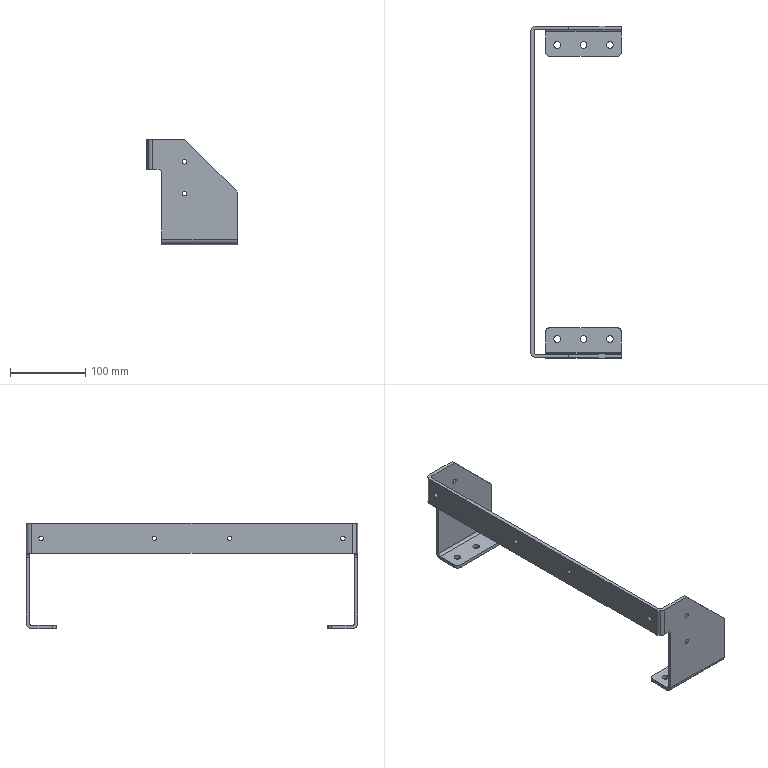Part | STEP file | STOPPER.BRACKET1.stp | 1 solid | 69 faces | box 120 x 440 x 140 mm | volume 215052 mm3 | cylinder 36 | spline 22 | plane 11 | commonest cylinder face diameters 6 x20 9 x6 10 x6 15 x4